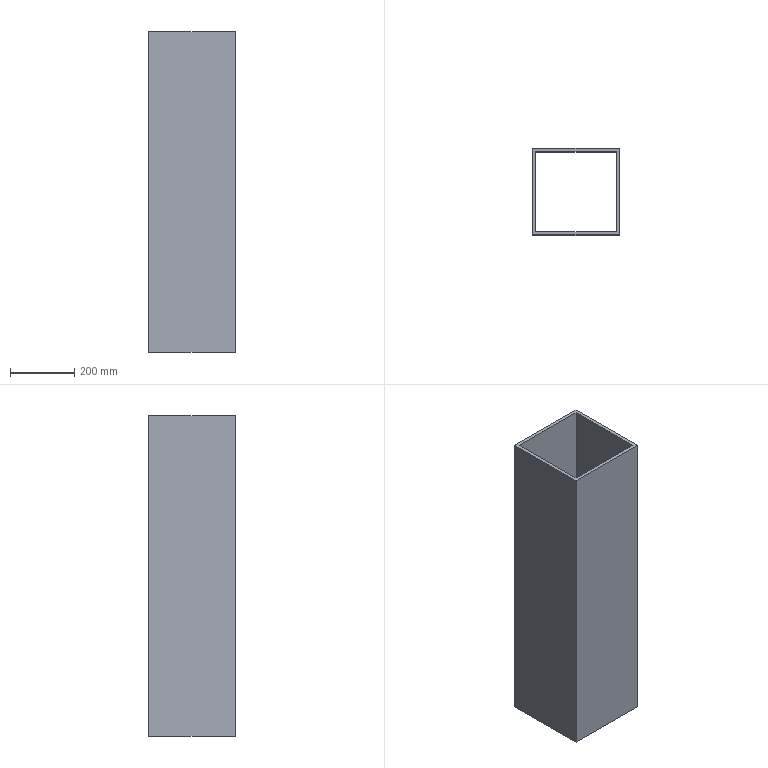Part | SolidWorks | features ExtruThin 1 | 1 solid | 10 faces | box 270 x 270 x 1000 mm | volume 10400000 mm3 | plane 10
STEP:
#1=CARTESIAN_POINT('',(-135.,135.,1000.));
#2=VERTEX_POINT('',#1);
#3=CARTESIAN_POINT('',(-135.,-135.,1000.));
#4=VERTEX_POINT('',#3);
#5=CARTESIAN_POINT('',(-135.,0.,1000.));
#6=DIRECTION('',(0.,-1.,0.));
#7=VECTOR('',#6,1000.);
#8=LINE('',#5,#7);
#9=EDGE_CURVE('',#2,#4,#8,.T.);
#10=ORIENTED_EDGE('',*,*,#9,.T.);
#11=CARTESIAN_POINT('',(135.,-135.,1000.));
#12=VERTEX_POINT('',#11);
#13=CARTESIAN_POINT('',(0.,-135.,1000.));
#14=DIRECTION('',(1.,0.,0.));
#15=VECTOR('',#14,1000.);
#16=LINE('',#13,#15);
#17=EDGE_CURVE('',#4,#12,#16,.T.);
#18=ORIENTED_EDGE('',*,*,#17,.T.);
#19=CARTESIAN_POINT('',(135.,135.,1000.));
#20=VERTEX_POINT('',#19);
#21=CARTESIAN_POINT('',(135.,0.,1000.));
#22=DIRECTION('',(0.,1.,0.));
#23=VECTOR('',#22,1000.);
#24=LINE('',#21,#23);
#25=EDGE_CURVE('',#12,#20,#24,.T.);
#26=ORIENTED_EDGE('',*,*,#25,.T.);
#27=CARTESIAN_POINT('',(0.,135.,1000.));
#28=DIRECTION('',(-1.,0.,0.));
#29=VECTOR('',#28,1000.);
#30=LINE('',#27,#29);
#31=EDGE_CURVE('',#20,#2,#30,.T.);
#32=ORIENTED_EDGE('',*,*,#31,.T.);
#33=EDGE_LOOP('',(#10,#18,#26,#32));
#34=FACE_OUTER_BOUND('',#33,.T.);
#35=CARTESIAN_POINT('',(-125.,-125.,1000.));
#36=VERTEX_POINT('',#35);
#37=CARTESIAN_POINT('',(125.,-125.,1000.));
#38=VERTEX_POINT('',#37);
#39=CARTESIAN_POINT('',(125.,-125.,1000.));
#40=DIRECTION('',(1.,0.,0.));
#41=VECTOR('',#40,1000.);
#42=LINE('',#39,#41);
#43=EDGE_CURVE('',#36,#38,#42,.T.);
#44=ORIENTED_EDGE('',*,*,#43,.F.);
#45=CARTESIAN_POINT('',(-125.,125.,1000.));
#46=VERTEX_POINT('',#45);
#47=CARTESIAN_POINT('',(-125.,125.,1000.));
#48=DIRECTION('',(0.,-1.,0.));
#49=VECTOR('',#48,1000.);
#50=LINE('',#47,#49);
#51=EDGE_CURVE('',#46,#36,#50,.T.);
#52=ORIENTED_EDGE('',*,*,#51,.F.);
#53=CARTESIAN_POINT('',(125.,125.,1000.));
#54=VERTEX_POINT('',#53);
#55=CARTESIAN_POINT('',(125.,125.,1000.));
#56=DIRECTION('',(-1.,0.,0.));
#57=VECTOR('',#56,1000.);
#58=LINE('',#55,#57);
#59=EDGE_CURVE('',#54,#46,#58,.T.);
#60=ORIENTED_EDGE('',*,*,#59,.F.);
#61=CARTESIAN_POINT('',(125.,125.,1000.));
#62=DIRECTION('',(0.,1.,0.));
#63=VECTOR('',#62,1000.);
#64=LINE('',#61,#63);
#65=EDGE_CURVE('',#38,#54,#64,.T.);
#66=ORIENTED_EDGE('',*,*,#65,.F.);
#67=EDGE_LOOP('',(#44,#52,#60,#66));
#68=FACE_BOUND('',#67,.T.);
#69=CARTESIAN_POINT('',(0.,0.,1000.));
#70=DIRECTION('',(0.,0.,1.));
#71=DIRECTION('',(1.,0.,0.));
#72=AXIS2_PLACEMENT_3D('',#69,#70,#71);
#73=PLANE('',#72);
#74=ADVANCED_FACE('',(#34,#68),#73,.T.);
#75=CARTESIAN_POINT('',(-135.,135.,0.));
#76=VERTEX_POINT('',#75);
#77=CARTESIAN_POINT('',(-135.,-135.,0.));
#78=VERTEX_POINT('',#77);
#79=CARTESIAN_POINT('',(-135.,0.,0.));
#80=DIRECTION('',(0.,-1.,0.));
#81=VECTOR('',#80,1000.);
#82=LINE('',#79,#81);
#83=EDGE_CURVE('',#76,#78,#82,.T.);
#84=ORIENTED_EDGE('',*,*,#83,.F.);
#85=CARTESIAN_POINT('',(135.,135.,0.));
#86=VERTEX_POINT('',#85);
#87=CARTESIAN_POINT('',(0.,135.,0.));
#88=DIRECTION('',(-1.,0.,0.));
#89=VECTOR('',#88,1000.);
#90=LINE('',#87,#89);
#91=EDGE_CURVE('',#86,#76,#90,.T.);
#92=ORIENTED_EDGE('',*,*,#91,.F.);
#93=CARTESIAN_POINT('',(135.,-135.,0.));
#94=VERTEX_POINT('',#93);
#95=CARTESIAN_POINT('',(135.,0.,0.));
#96=DIRECTION('',(0.,1.,0.));
#97=VECTOR('',#96,1000.);
#98=LINE('',#95,#97);
#99=EDGE_CURVE('',#94,#86,#98,.T.);
#100=ORIENTED_EDGE('',*,*,#99,.F.);
#101=CARTESIAN_POINT('',(0.,-135.,0.));
#102=DIRECTION('',(1.,0.,0.));
#103=VECTOR('',#102,1000.);
#104=LINE('',#101,#103);
#105=EDGE_CURVE('',#78,#94,#104,.T.);
#106=ORIENTED_EDGE('',*,*,#105,.F.);
#107=EDGE_LOOP('',(#84,#92,#100,#106));
#108=FACE_OUTER_BOUND('',#107,.T.);
#109=CARTESIAN_POINT('',(-125.,125.,0.));
#110=VERTEX_POINT('',#109);
#111=CARTESIAN_POINT('',(-125.,-125.,0.));
#112=VERTEX_POINT('',#111);
#113=CARTESIAN_POINT('',(-125.,125.,0.));
#114=DIRECTION('',(0.,-1.,0.));
#115=VECTOR('',#114,1000.);
#116=LINE('',#113,#115);
#117=EDGE_CURVE('',#110,#112,#116,.T.);
#118=ORIENTED_EDGE('',*,*,#117,.T.);
#119=CARTESIAN_POINT('',(125.,-125.,0.));
#120=VERTEX_POINT('',#119);
#121=CARTESIAN_POINT('',(125.,-125.,0.));
#122=DIRECTION('',(1.,0.,0.));
#123=VECTOR('',#122,1000.);
#124=LINE('',#121,#123);
#125=EDGE_CURVE('',#112,#120,#124,.T.);
#126=ORIENTED_EDGE('',*,*,#125,.T.);
#127=CARTESIAN_POINT('',(125.,125.,0.));
#128=VERTEX_POINT('',#127);
#129=CARTESIAN_POINT('',(125.,125.,0.));
#130=DIRECTION('',(0.,1.,0.));
#131=VECTOR('',#130,1000.);
#132=LINE('',#129,#131);
#133=EDGE_CURVE('',#120,#128,#132,.T.);
#134=ORIENTED_EDGE('',*,*,#133,.T.);
#135=CARTESIAN_POINT('',(125.,125.,0.));
#136=DIRECTION('',(-1.,0.,0.));
#137=VECTOR('',#136,1000.);
#138=LINE('',#135,#137);
#139=EDGE_CURVE('',#128,#110,#138,.T.);
#140=ORIENTED_EDGE('',*,*,#139,.T.);
#141=EDGE_LOOP('',(#118,#126,#134,#140));
#142=FACE_BOUND('',#141,.T.);
#143=CARTESIAN_POINT('',(0.,0.,0.));
#144=DIRECTION('',(0.,0.,1.));
#145=DIRECTION('',(1.,0.,0.));
#146=AXIS2_PLACEMENT_3D('',#143,#144,#145);
#147=PLANE('',#146);
#148=ADVANCED_FACE('',(#108,#142),#147,.F.);
#149=ORIENTED_EDGE('',*,*,#83,.T.);
#150=CARTESIAN_POINT('',(-135.,-135.,1000.));
#151=DIRECTION('',(0.,0.,-1.));
#152=VECTOR('',#151,1000.);
#153=LINE('',#150,#152);
#154=EDGE_CURVE('',#4,#78,#153,.T.);
#155=ORIENTED_EDGE('',*,*,#154,.F.);
#156=ORIENTED_EDGE('',*,*,#9,.F.);
#157=CARTESIAN_POINT('',(-135.,135.,1000.));
#158=DIRECTION('',(0.,0.,-1.));
#159=VECTOR('',#158,1000.);
#160=LINE('',#157,#159);
#161=EDGE_CURVE('',#2,#76,#160,.T.);
#162=ORIENTED_EDGE('',*,*,#161,.T.);
#163=EDGE_LOOP('',(#149,#155,#156,#162));
#164=FACE_OUTER_BOUND('',#163,.T.);
#165=CARTESIAN_POINT('',(-135.,0.,1000.));
#166=DIRECTION('',(1.,0.,0.));
#167=DIRECTION('',(0.,1.,0.));
#168=AXIS2_PLACEMENT_3D('',#165,#166,#167);
#169=PLANE('',#168);
#170=ADVANCED_FACE('',(#164),#169,.F.);
#171=ORIENTED_EDGE('',*,*,#105,.T.);
#172=CARTESIAN_POINT('',(135.,-135.,1000.));
#173=DIRECTION('',(0.,0.,-1.));
#174=VECTOR('',#173,1000.);
#175=LINE('',#172,#174);
#176=EDGE_CURVE('',#12,#94,#175,.T.);
#177=ORIENTED_EDGE('',*,*,#176,.F.);
#178=ORIENTED_EDGE('',*,*,#17,.F.);
#179=ORIENTED_EDGE('',*,*,#154,.T.);
#180=EDGE_LOOP('',(#171,#177,#178,#179));
#181=FACE_OUTER_BOUND('',#180,.T.);
#182=CARTESIAN_POINT('',(0.,-135.,1000.));
#183=DIRECTION('',(0.,1.,0.));
#184=DIRECTION('',(-1.,0.,0.));
#185=AXIS2_PLACEMENT_3D('',#182,#183,#184);
#186=PLANE('',#185);
#187=ADVANCED_FACE('',(#181),#186,.F.);
#188=ORIENTED_EDGE('',*,*,#99,.T.);
#189=CARTESIAN_POINT('',(135.,135.,1000.));
#190=DIRECTION('',(0.,0.,-1.));
#191=VECTOR('',#190,1000.);
#192=LINE('',#189,#191);
#193=EDGE_CURVE('',#20,#86,#192,.T.);
#194=ORIENTED_EDGE('',*,*,#193,.F.);
#195=ORIENTED_EDGE('',*,*,#25,.F.);
#196=ORIENTED_EDGE('',*,*,#176,.T.);
#197=EDGE_LOOP('',(#188,#194,#195,#196));
#198=FACE_OUTER_BOUND('',#197,.T.);
#199=CARTESIAN_POINT('',(135.,0.,1000.));
#200=DIRECTION('',(-1.,0.,0.));
#201=DIRECTION('',(0.,-1.,0.));
#202=AXIS2_PLACEMENT_3D('',#199,#200,#201);
#203=PLANE('',#202);
#204=ADVANCED_FACE('',(#198),#203,.F.);
#205=ORIENTED_EDGE('',*,*,#91,.T.);
#206=ORIENTED_EDGE('',*,*,#161,.F.);
#207=ORIENTED_EDGE('',*,*,#31,.F.);
#208=ORIENTED_EDGE('',*,*,#193,.T.);
#209=EDGE_LOOP('',(#205,#206,#207,#208));
#210=FACE_OUTER_BOUND('',#209,.T.);
#211=CARTESIAN_POINT('',(0.,135.,1000.));
#212=DIRECTION('',(0.,-1.,0.));
#213=DIRECTION('',(1.,0.,0.));
#214=AXIS2_PLACEMENT_3D('',#211,#212,#213);
#215=PLANE('',#214);
#216=ADVANCED_FACE('',(#210),#215,.F.);
#217=ORIENTED_EDGE('',*,*,#117,.F.);
#218=CARTESIAN_POINT('',(-125.,125.,1000.));
#219=DIRECTION('',(0.,0.,-1.));
#220=VECTOR('',#219,1000.);
#221=LINE('',#218,#220);
#222=EDGE_CURVE('',#46,#110,#221,.T.);
#223=ORIENTED_EDGE('',*,*,#222,.F.);
#224=ORIENTED_EDGE('',*,*,#51,.T.);
#225=CARTESIAN_POINT('',(-125.,-125.,1000.));
#226=DIRECTION('',(0.,0.,-1.));
#227=VECTOR('',#226,1000.);
#228=LINE('',#225,#227);
#229=EDGE_CURVE('',#36,#112,#228,.T.);
#230=ORIENTED_EDGE('',*,*,#229,.T.);
#231=EDGE_LOOP('',(#217,#223,#224,#230));
#232=FACE_OUTER_BOUND('',#231,.T.);
#233=CARTESIAN_POINT('',(-125.,125.,1000.));
#234=DIRECTION('',(1.,0.,0.));
#235=DIRECTION('',(0.,1.,0.));
#236=AXIS2_PLACEMENT_3D('',#233,#234,#235);
#237=PLANE('',#236);
#238=ADVANCED_FACE('',(#232),#237,.T.);
#239=ORIENTED_EDGE('',*,*,#125,.F.);
#240=ORIENTED_EDGE('',*,*,#229,.F.);
#241=ORIENTED_EDGE('',*,*,#43,.T.);
#242=CARTESIAN_POINT('',(125.,-125.,1000.));
#243=DIRECTION('',(0.,0.,-1.));
#244=VECTOR('',#243,1000.);
#245=LINE('',#242,#244);
#246=EDGE_CURVE('',#38,#120,#245,.T.);
#247=ORIENTED_EDGE('',*,*,#246,.T.);
#248=EDGE_LOOP('',(#239,#240,#241,#247));
#249=FACE_OUTER_BOUND('',#248,.T.);
#250=CARTESIAN_POINT('',(125.,-125.,1000.));
#251=DIRECTION('',(0.,1.,0.));
#252=DIRECTION('',(-1.,0.,0.));
#253=AXIS2_PLACEMENT_3D('',#250,#251,#252);
#254=PLANE('',#253);
#255=ADVANCED_FACE('',(#249),#254,.T.);
#256=ORIENTED_EDGE('',*,*,#133,.F.);
#257=ORIENTED_EDGE('',*,*,#246,.F.);
#258=ORIENTED_EDGE('',*,*,#65,.T.);
#259=CARTESIAN_POINT('',(125.,125.,1000.));
#260=DIRECTION('',(0.,0.,-1.));
#261=VECTOR('',#260,1000.);
#262=LINE('',#259,#261);
#263=EDGE_CURVE('',#54,#128,#262,.T.);
#264=ORIENTED_EDGE('',*,*,#263,.T.);
#265=EDGE_LOOP('',(#256,#257,#258,#264));
#266=FACE_OUTER_BOUND('',#265,.T.);
#267=CARTESIAN_POINT('',(125.,125.,1000.));
#268=DIRECTION('',(-1.,0.,0.));
#269=DIRECTION('',(0.,-1.,0.));
#270=AXIS2_PLACEMENT_3D('',#267,#268,#269);
#271=PLANE('',#270);
#272=ADVANCED_FACE('',(#266),#271,.T.);
#273=ORIENTED_EDGE('',*,*,#139,.F.);
#274=ORIENTED_EDGE('',*,*,#263,.F.);
#275=ORIENTED_EDGE('',*,*,#59,.T.);
#276=ORIENTED_EDGE('',*,*,#222,.T.);
#277=EDGE_LOOP('',(#273,#274,#275,#276));
#278=FACE_OUTER_BOUND('',#277,.T.);
#279=CARTESIAN_POINT('',(125.,125.,1000.));
#280=DIRECTION('',(0.,-1.,0.));
#281=DIRECTION('',(1.,0.,0.));
#282=AXIS2_PLACEMENT_3D('',#279,#280,#281);
#283=PLANE('',#282);
#284=ADVANCED_FACE('',(#278),#283,.T.);
#285=CLOSED_SHELL('',(#74,#148,#170,#187,#204,#216,#238,#255,#272,#284));
#286=MANIFOLD_SOLID_BREP('',#285);
#287=CARTESIAN_POINT('',(0.,0.,0.));
#288=DIRECTION('',(0.,0.,1.));
#289=DIRECTION('',(1.,0.,0.));
#290=AXIS2_PLACEMENT_3D('',#287,#288,#289);
#291=(LENGTH_UNIT()NAMED_UNIT(*)SI_UNIT(.MILLI.,.METRE.));
#292=UNCERTAINTY_MEASURE_WITH_UNIT(LENGTH_MEASURE(0.00001),#291,'','');
#293=(NAMED_UNIT(*)PLANE_ANGLE_UNIT()SI_UNIT($,.RADIAN.));
#294=(NAMED_UNIT(*)SI_UNIT($,.STERADIAN.)SOLID_ANGLE_UNIT());
#295=(GEOMETRIC_REPRESENTATION_CONTEXT(3)GLOBAL_UNCERTAINTY_ASSIGNED_CONTEXT((#292))GLOBAL_UNIT_ASSIGNED_CONTEXT((#291,#293,#294))REPRESENTATION_CONTEXT('',''));
#296=ADVANCED_BREP_SHAPE_REPRESENTATION('',(#286,#290),#295);